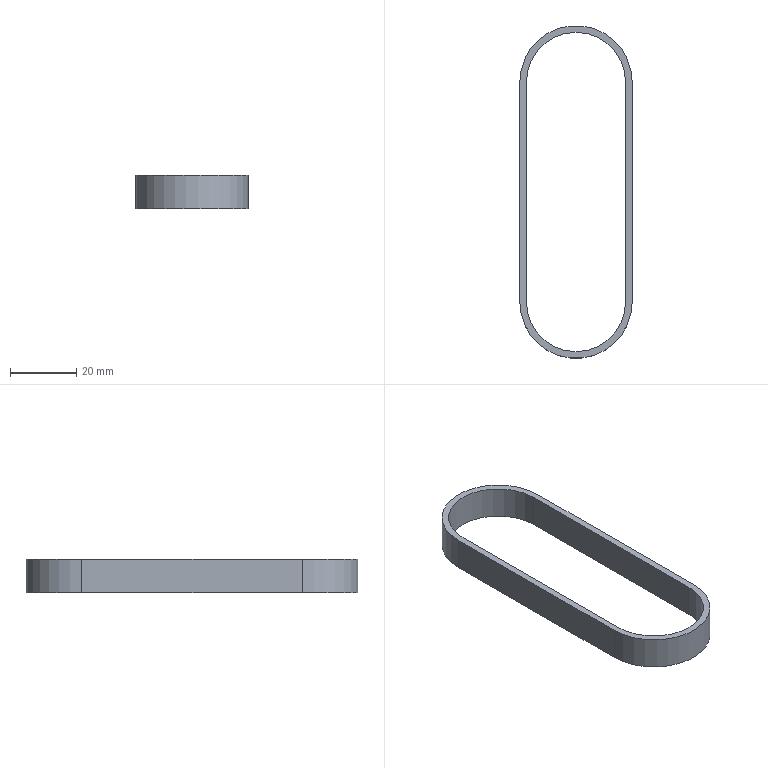Part | SolidWorks | features BeltProfileFeature 1, ExtruThin 1 | 1 solid | 10 faces | box 33.89 x 100.315 x 10 mm | volume 4661 mm3 | plane 6 | cylinder 4 | commonest cylinder face diameters 29.89 x2 33.89 x2
STEP:
#1=CARTESIAN_POINT('',(3.548,-3.001,10.));
#2=VERTEX_POINT('',#1);
#3=CARTESIAN_POINT('',(-30.342,-3.001,10.));
#4=VERTEX_POINT('',#3);
#5=CARTESIAN_POINT('',(-13.397,-3.001,10.));
#6=DIRECTION('',(0.,0.,1.));
#7=DIRECTION('',(-1.,0.,0.));
#8=AXIS2_PLACEMENT_3D('',#5,#6,#7);
#9=CIRCLE('',#8,16.945);
#10=EDGE_CURVE('',#2,#4,#9,.T.);
#11=ORIENTED_EDGE('',*,*,#10,.T.);
#12=CARTESIAN_POINT('',(-30.342,-69.426,10.));
#13=VERTEX_POINT('',#12);
#14=CARTESIAN_POINT('',(-30.342,-69.426,10.));
#15=DIRECTION('',(0.,-1.,0.));
#16=VECTOR('',#15,1000.);
#17=LINE('',#14,#16);
#18=EDGE_CURVE('',#4,#13,#17,.T.);
#19=ORIENTED_EDGE('',*,*,#18,.T.);
#20=CARTESIAN_POINT('',(3.548,-69.426,10.));
#21=VERTEX_POINT('',#20);
#22=CARTESIAN_POINT('',(-13.397,-69.426,10.));
#23=DIRECTION('',(0.,0.,1.));
#24=DIRECTION('',(-1.,0.,0.));
#25=AXIS2_PLACEMENT_3D('',#22,#23,#24);
#26=CIRCLE('',#25,16.945);
#27=EDGE_CURVE('',#13,#21,#26,.T.);
#28=ORIENTED_EDGE('',*,*,#27,.T.);
#29=CARTESIAN_POINT('',(3.548,-3.001,10.));
#30=DIRECTION('',(0.,1.,0.));
#31=VECTOR('',#30,1000.);
#32=LINE('',#29,#31);
#33=EDGE_CURVE('',#21,#2,#32,.T.);
#34=ORIENTED_EDGE('',*,*,#33,.T.);
#35=EDGE_LOOP('',(#11,#19,#28,#34));
#36=FACE_OUTER_BOUND('',#35,.T.);
#37=CARTESIAN_POINT('',(-28.342,-3.001,10.));
#38=VERTEX_POINT('',#37);
#39=CARTESIAN_POINT('',(-28.342,-69.426,10.));
#40=VERTEX_POINT('',#39);
#41=CARTESIAN_POINT('',(-28.342,-3.001,10.));
#42=DIRECTION('',(0.,-1.,0.));
#43=VECTOR('',#42,1000.);
#44=LINE('',#41,#43);
#45=EDGE_CURVE('',#38,#40,#44,.T.);
#46=ORIENTED_EDGE('',*,*,#45,.F.);
#47=CARTESIAN_POINT('',(1.548,-3.001,10.));
#48=VERTEX_POINT('',#47);
#49=CARTESIAN_POINT('',(-13.397,-3.001,10.));
#50=DIRECTION('',(0.,0.,1.));
#51=DIRECTION('',(-1.,0.,0.));
#52=AXIS2_PLACEMENT_3D('',#49,#50,#51);
#53=CIRCLE('',#52,14.945);
#54=EDGE_CURVE('',#48,#38,#53,.T.);
#55=ORIENTED_EDGE('',*,*,#54,.F.);
#56=CARTESIAN_POINT('',(1.548,-69.426,10.));
#57=VERTEX_POINT('',#56);
#58=CARTESIAN_POINT('',(1.548,-3.001,10.));
#59=DIRECTION('',(0.,1.,0.));
#60=VECTOR('',#59,1000.);
#61=LINE('',#58,#60);
#62=EDGE_CURVE('',#57,#48,#61,.T.);
#63=ORIENTED_EDGE('',*,*,#62,.F.);
#64=CARTESIAN_POINT('',(-13.397,-69.426,10.));
#65=DIRECTION('',(0.,0.,1.));
#66=DIRECTION('',(-1.,0.,0.));
#67=AXIS2_PLACEMENT_3D('',#64,#65,#66);
#68=CIRCLE('',#67,14.945);
#69=EDGE_CURVE('',#40,#57,#68,.T.);
#70=ORIENTED_EDGE('',*,*,#69,.F.);
#71=EDGE_LOOP('',(#46,#55,#63,#70));
#72=FACE_BOUND('',#71,.T.);
#73=CARTESIAN_POINT('',(-13.397,-3.001,10.));
#74=DIRECTION('',(0.,0.,1.));
#75=DIRECTION('',(1.,0.,0.));
#76=AXIS2_PLACEMENT_3D('',#73,#74,#75);
#77=PLANE('',#76);
#78=ADVANCED_FACE('',(#36,#72),#77,.T.);
#79=CARTESIAN_POINT('',(3.548,-3.001,0.));
#80=VERTEX_POINT('',#79);
#81=CARTESIAN_POINT('',(-30.342,-3.001,0.));
#82=VERTEX_POINT('',#81);
#83=CARTESIAN_POINT('',(-13.397,-3.001,0.));
#84=DIRECTION('',(0.,0.,1.));
#85=DIRECTION('',(-1.,0.,0.));
#86=AXIS2_PLACEMENT_3D('',#83,#84,#85);
#87=CIRCLE('',#86,16.945);
#88=EDGE_CURVE('',#80,#82,#87,.T.);
#89=ORIENTED_EDGE('',*,*,#88,.F.);
#90=CARTESIAN_POINT('',(3.548,-69.426,0.));
#91=VERTEX_POINT('',#90);
#92=CARTESIAN_POINT('',(3.548,-3.001,0.));
#93=DIRECTION('',(0.,1.,0.));
#94=VECTOR('',#93,1000.);
#95=LINE('',#92,#94);
#96=EDGE_CURVE('',#91,#80,#95,.T.);
#97=ORIENTED_EDGE('',*,*,#96,.F.);
#98=CARTESIAN_POINT('',(-30.342,-69.426,0.));
#99=VERTEX_POINT('',#98);
#100=CARTESIAN_POINT('',(-13.397,-69.426,0.));
#101=DIRECTION('',(0.,0.,1.));
#102=DIRECTION('',(-1.,0.,0.));
#103=AXIS2_PLACEMENT_3D('',#100,#101,#102);
#104=CIRCLE('',#103,16.945);
#105=EDGE_CURVE('',#99,#91,#104,.T.);
#106=ORIENTED_EDGE('',*,*,#105,.F.);
#107=CARTESIAN_POINT('',(-30.342,-69.426,0.));
#108=DIRECTION('',(0.,-1.,0.));
#109=VECTOR('',#108,1000.);
#110=LINE('',#107,#109);
#111=EDGE_CURVE('',#82,#99,#110,.T.);
#112=ORIENTED_EDGE('',*,*,#111,.F.);
#113=EDGE_LOOP('',(#89,#97,#106,#112));
#114=FACE_OUTER_BOUND('',#113,.T.);
#115=CARTESIAN_POINT('',(1.548,-3.001,0.));
#116=VERTEX_POINT('',#115);
#117=CARTESIAN_POINT('',(-28.342,-3.001,0.));
#118=VERTEX_POINT('',#117);
#119=CARTESIAN_POINT('',(-13.397,-3.001,0.));
#120=DIRECTION('',(0.,0.,1.));
#121=DIRECTION('',(-1.,0.,0.));
#122=AXIS2_PLACEMENT_3D('',#119,#120,#121);
#123=CIRCLE('',#122,14.945);
#124=EDGE_CURVE('',#116,#118,#123,.T.);
#125=ORIENTED_EDGE('',*,*,#124,.T.);
#126=CARTESIAN_POINT('',(-28.342,-69.426,0.));
#127=VERTEX_POINT('',#126);
#128=CARTESIAN_POINT('',(-28.342,-3.001,0.));
#129=DIRECTION('',(0.,-1.,0.));
#130=VECTOR('',#129,1000.);
#131=LINE('',#128,#130);
#132=EDGE_CURVE('',#118,#127,#131,.T.);
#133=ORIENTED_EDGE('',*,*,#132,.T.);
#134=CARTESIAN_POINT('',(1.548,-69.426,0.));
#135=VERTEX_POINT('',#134);
#136=CARTESIAN_POINT('',(-13.397,-69.426,0.));
#137=DIRECTION('',(0.,0.,1.));
#138=DIRECTION('',(-1.,0.,0.));
#139=AXIS2_PLACEMENT_3D('',#136,#137,#138);
#140=CIRCLE('',#139,14.945);
#141=EDGE_CURVE('',#127,#135,#140,.T.);
#142=ORIENTED_EDGE('',*,*,#141,.T.);
#143=CARTESIAN_POINT('',(1.548,-3.001,0.));
#144=DIRECTION('',(0.,1.,0.));
#145=VECTOR('',#144,1000.);
#146=LINE('',#143,#145);
#147=EDGE_CURVE('',#135,#116,#146,.T.);
#148=ORIENTED_EDGE('',*,*,#147,.T.);
#149=EDGE_LOOP('',(#125,#133,#142,#148));
#150=FACE_BOUND('',#149,.T.);
#151=CARTESIAN_POINT('',(-13.397,-3.001,0.));
#152=DIRECTION('',(0.,0.,1.));
#153=DIRECTION('',(1.,0.,0.));
#154=AXIS2_PLACEMENT_3D('',#151,#152,#153);
#155=PLANE('',#154);
#156=ADVANCED_FACE('',(#114,#150),#155,.F.);
#157=ORIENTED_EDGE('',*,*,#88,.T.);
#158=CARTESIAN_POINT('',(-30.342,-3.001,10.));
#159=DIRECTION('',(0.,0.,-1.));
#160=VECTOR('',#159,1000.);
#161=LINE('',#158,#160);
#162=EDGE_CURVE('',#4,#82,#161,.T.);
#163=ORIENTED_EDGE('',*,*,#162,.F.);
#164=ORIENTED_EDGE('',*,*,#10,.F.);
#165=CARTESIAN_POINT('',(3.548,-3.001,10.));
#166=DIRECTION('',(0.,0.,-1.));
#167=VECTOR('',#166,1000.);
#168=LINE('',#165,#167);
#169=EDGE_CURVE('',#2,#80,#168,.T.);
#170=ORIENTED_EDGE('',*,*,#169,.T.);
#171=EDGE_LOOP('',(#157,#163,#164,#170));
#172=FACE_OUTER_BOUND('',#171,.T.);
#173=CARTESIAN_POINT('',(-13.397,-3.001,10.));
#174=DIRECTION('',(0.,0.,-1.));
#175=DIRECTION('',(-1.,0.,0.));
#176=AXIS2_PLACEMENT_3D('',#173,#174,#175);
#177=CYLINDRICAL_SURFACE('',#176,16.945);
#178=ADVANCED_FACE('',(#172),#177,.T.);
#179=ORIENTED_EDGE('',*,*,#111,.T.);
#180=CARTESIAN_POINT('',(-30.342,-69.426,10.));
#181=DIRECTION('',(0.,0.,-1.));
#182=VECTOR('',#181,1000.);
#183=LINE('',#180,#182);
#184=EDGE_CURVE('',#13,#99,#183,.T.);
#185=ORIENTED_EDGE('',*,*,#184,.F.);
#186=ORIENTED_EDGE('',*,*,#18,.F.);
#187=ORIENTED_EDGE('',*,*,#162,.T.);
#188=EDGE_LOOP('',(#179,#185,#186,#187));
#189=FACE_OUTER_BOUND('',#188,.T.);
#190=CARTESIAN_POINT('',(-30.342,-69.426,10.));
#191=DIRECTION('',(1.,0.,0.));
#192=DIRECTION('',(0.,0.,-1.));
#193=AXIS2_PLACEMENT_3D('',#190,#191,#192);
#194=PLANE('',#193);
#195=ADVANCED_FACE('',(#189),#194,.F.);
#196=ORIENTED_EDGE('',*,*,#105,.T.);
#197=CARTESIAN_POINT('',(3.548,-69.426,10.));
#198=DIRECTION('',(0.,0.,-1.));
#199=VECTOR('',#198,1000.);
#200=LINE('',#197,#199);
#201=EDGE_CURVE('',#21,#91,#200,.T.);
#202=ORIENTED_EDGE('',*,*,#201,.F.);
#203=ORIENTED_EDGE('',*,*,#27,.F.);
#204=ORIENTED_EDGE('',*,*,#184,.T.);
#205=EDGE_LOOP('',(#196,#202,#203,#204));
#206=FACE_OUTER_BOUND('',#205,.T.);
#207=CARTESIAN_POINT('',(-13.397,-69.426,10.));
#208=DIRECTION('',(0.,0.,-1.));
#209=DIRECTION('',(-1.,0.,0.));
#210=AXIS2_PLACEMENT_3D('',#207,#208,#209);
#211=CYLINDRICAL_SURFACE('',#210,16.945);
#212=ADVANCED_FACE('',(#206),#211,.T.);
#213=ORIENTED_EDGE('',*,*,#96,.T.);
#214=ORIENTED_EDGE('',*,*,#169,.F.);
#215=ORIENTED_EDGE('',*,*,#33,.F.);
#216=ORIENTED_EDGE('',*,*,#201,.T.);
#217=EDGE_LOOP('',(#213,#214,#215,#216));
#218=FACE_OUTER_BOUND('',#217,.T.);
#219=CARTESIAN_POINT('',(3.548,-3.001,10.));
#220=DIRECTION('',(-1.,0.,0.));
#221=DIRECTION('',(0.,0.,1.));
#222=AXIS2_PLACEMENT_3D('',#219,#220,#221);
#223=PLANE('',#222);
#224=ADVANCED_FACE('',(#218),#223,.F.);
#225=ORIENTED_EDGE('',*,*,#124,.F.);
#226=CARTESIAN_POINT('',(1.548,-3.001,10.));
#227=DIRECTION('',(0.,0.,-1.));
#228=VECTOR('',#227,1000.);
#229=LINE('',#226,#228);
#230=EDGE_CURVE('',#48,#116,#229,.T.);
#231=ORIENTED_EDGE('',*,*,#230,.F.);
#232=ORIENTED_EDGE('',*,*,#54,.T.);
#233=CARTESIAN_POINT('',(-28.342,-3.001,10.));
#234=DIRECTION('',(0.,0.,-1.));
#235=VECTOR('',#234,1000.);
#236=LINE('',#233,#235);
#237=EDGE_CURVE('',#38,#118,#236,.T.);
#238=ORIENTED_EDGE('',*,*,#237,.T.);
#239=EDGE_LOOP('',(#225,#231,#232,#238));
#240=FACE_OUTER_BOUND('',#239,.T.);
#241=CARTESIAN_POINT('',(-13.397,-3.001,10.));
#242=DIRECTION('',(0.,0.,-1.));
#243=DIRECTION('',(-1.,0.,0.));
#244=AXIS2_PLACEMENT_3D('',#241,#242,#243);
#245=CYLINDRICAL_SURFACE('',#244,14.945);
#246=ADVANCED_FACE('',(#240),#245,.F.);
#247=ORIENTED_EDGE('',*,*,#132,.F.);
#248=ORIENTED_EDGE('',*,*,#237,.F.);
#249=ORIENTED_EDGE('',*,*,#45,.T.);
#250=CARTESIAN_POINT('',(-28.342,-69.426,10.));
#251=DIRECTION('',(0.,0.,-1.));
#252=VECTOR('',#251,1000.);
#253=LINE('',#250,#252);
#254=EDGE_CURVE('',#40,#127,#253,.T.);
#255=ORIENTED_EDGE('',*,*,#254,.T.);
#256=EDGE_LOOP('',(#247,#248,#249,#255));
#257=FACE_OUTER_BOUND('',#256,.T.);
#258=CARTESIAN_POINT('',(-28.342,-3.001,10.));
#259=DIRECTION('',(1.,0.,0.));
#260=DIRECTION('',(0.,0.,-1.));
#261=AXIS2_PLACEMENT_3D('',#258,#259,#260);
#262=PLANE('',#261);
#263=ADVANCED_FACE('',(#257),#262,.T.);
#264=ORIENTED_EDGE('',*,*,#141,.F.);
#265=ORIENTED_EDGE('',*,*,#254,.F.);
#266=ORIENTED_EDGE('',*,*,#69,.T.);
#267=CARTESIAN_POINT('',(1.548,-69.426,10.));
#268=DIRECTION('',(0.,0.,-1.));
#269=VECTOR('',#268,1000.);
#270=LINE('',#267,#269);
#271=EDGE_CURVE('',#57,#135,#270,.T.);
#272=ORIENTED_EDGE('',*,*,#271,.T.);
#273=EDGE_LOOP('',(#264,#265,#266,#272));
#274=FACE_OUTER_BOUND('',#273,.T.);
#275=CARTESIAN_POINT('',(-13.397,-69.426,10.));
#276=DIRECTION('',(0.,0.,-1.));
#277=DIRECTION('',(-1.,0.,0.));
#278=AXIS2_PLACEMENT_3D('',#275,#276,#277);
#279=CYLINDRICAL_SURFACE('',#278,14.945);
#280=ADVANCED_FACE('',(#274),#279,.F.);
#281=ORIENTED_EDGE('',*,*,#147,.F.);
#282=ORIENTED_EDGE('',*,*,#271,.F.);
#283=ORIENTED_EDGE('',*,*,#62,.T.);
#284=ORIENTED_EDGE('',*,*,#230,.T.);
#285=EDGE_LOOP('',(#281,#282,#283,#284));
#286=FACE_OUTER_BOUND('',#285,.T.);
#287=CARTESIAN_POINT('',(1.548,-3.001,10.));
#288=DIRECTION('',(-1.,0.,0.));
#289=DIRECTION('',(0.,0.,1.));
#290=AXIS2_PLACEMENT_3D('',#287,#288,#289);
#291=PLANE('',#290);
#292=ADVANCED_FACE('',(#286),#291,.T.);
#293=CLOSED_SHELL('',(#78,#156,#178,#195,#212,#224,#246,#263,#280,#292));
#294=MANIFOLD_SOLID_BREP('',#293);
#295=CARTESIAN_POINT('',(0.,0.,0.));
#296=DIRECTION('',(0.,0.,1.));
#297=DIRECTION('',(1.,0.,0.));
#298=AXIS2_PLACEMENT_3D('',#295,#296,#297);
#299=(LENGTH_UNIT()NAMED_UNIT(*)SI_UNIT(.MILLI.,.METRE.));
#300=UNCERTAINTY_MEASURE_WITH_UNIT(LENGTH_MEASURE(0.00001),#299,'','');
#301=(NAMED_UNIT(*)PLANE_ANGLE_UNIT()SI_UNIT($,.RADIAN.));
#302=(NAMED_UNIT(*)SI_UNIT($,.STERADIAN.)SOLID_ANGLE_UNIT());
#303=(GEOMETRIC_REPRESENTATION_CONTEXT(3)GLOBAL_UNCERTAINTY_ASSIGNED_CONTEXT((#300))GLOBAL_UNIT_ASSIGNED_CONTEXT((#299,#301,#302))REPRESENTATION_CONTEXT('',''));
#304=ADVANCED_BREP_SHAPE_REPRESENTATION('',(#294,#298),#303);